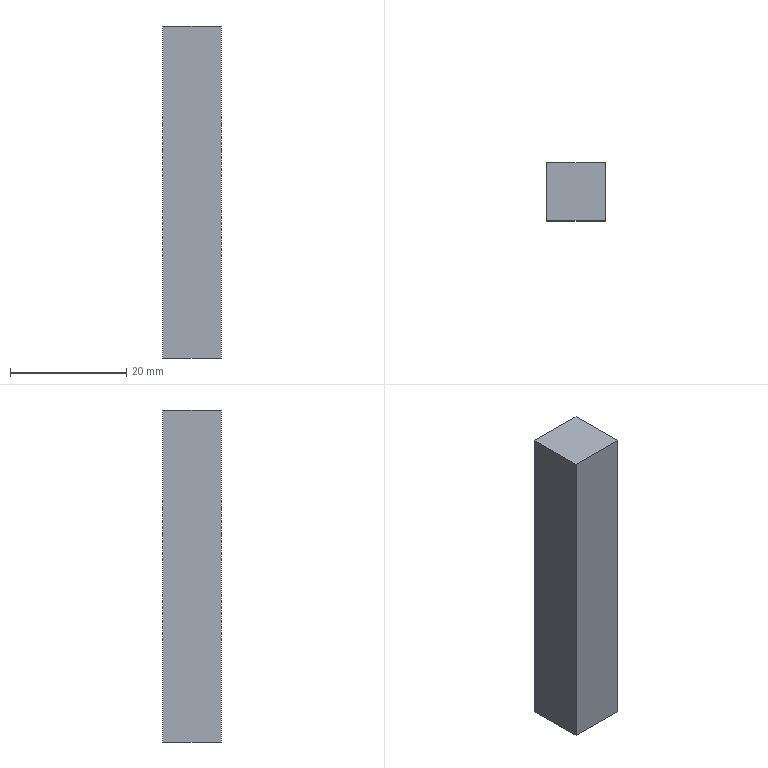Part | NX | features BREP 1 | 1 solid | 6 faces | box 10 x 10 x 57 mm | volume 5700 mm3 | plane 6
STEP:
#1=CARTESIAN_POINT('',(-1.25,10.55,-5.));
#2=VERTEX_POINT('',#1);
#3=CARTESIAN_POINT('',(-1.25,0.55,-5.));
#4=VERTEX_POINT('',#3);
#5=CARTESIAN_POINT('',(-1.25,10.55,-5.));
#6=DIRECTION('',(0.,-1.,0.));
#7=VECTOR('',#6,1000.);
#8=LINE('',#5,#7);
#9=EDGE_CURVE('',#2,#4,#8,.T.);
#10=ORIENTED_EDGE('',*,*,#9,.T.);
#11=CARTESIAN_POINT('',(-1.25,0.55,52.));
#12=VERTEX_POINT('',#11);
#13=CARTESIAN_POINT('',(-1.25,0.55,52.));
#14=DIRECTION('',(0.,0.,-1.));
#15=VECTOR('',#14,1000.);
#16=LINE('',#13,#15);
#17=EDGE_CURVE('',#12,#4,#16,.T.);
#18=ORIENTED_EDGE('',*,*,#17,.F.);
#19=CARTESIAN_POINT('',(-1.25,10.55,52.));
#20=VERTEX_POINT('',#19);
#21=CARTESIAN_POINT('',(-1.25,10.55,52.));
#22=DIRECTION('',(0.,-1.,0.));
#23=VECTOR('',#22,1000.);
#24=LINE('',#21,#23);
#25=EDGE_CURVE('',#20,#12,#24,.T.);
#26=ORIENTED_EDGE('',*,*,#25,.F.);
#27=CARTESIAN_POINT('',(-1.25,10.55,52.));
#28=DIRECTION('',(0.,0.,-1.));
#29=VECTOR('',#28,1000.);
#30=LINE('',#27,#29);
#31=EDGE_CURVE('',#20,#2,#30,.T.);
#32=ORIENTED_EDGE('',*,*,#31,.T.);
#33=EDGE_LOOP('',(#10,#18,#26,#32));
#34=FACE_BOUND('',#33,.T.);
#35=CARTESIAN_POINT('',(-1.25,10.55,52.));
#36=DIRECTION('',(1.,0.,0.));
#37=DIRECTION('',(0.,0.,1.));
#38=AXIS2_PLACEMENT_3D('',#35,#36,#37);
#39=PLANE('',#38);
#40=ADVANCED_FACE('',(#34),#39,.F.);
#41=CARTESIAN_POINT('',(8.75,0.55,-5.));
#42=VERTEX_POINT('',#41);
#43=CARTESIAN_POINT('',(-1.25,0.55,-5.));
#44=DIRECTION('',(1.,0.,0.));
#45=VECTOR('',#44,1000.);
#46=LINE('',#43,#45);
#47=EDGE_CURVE('',#4,#42,#46,.T.);
#48=ORIENTED_EDGE('',*,*,#47,.T.);
#49=CARTESIAN_POINT('',(8.75,0.55,52.));
#50=VERTEX_POINT('',#49);
#51=CARTESIAN_POINT('',(8.75,0.55,52.));
#52=DIRECTION('',(0.,0.,-1.));
#53=VECTOR('',#52,1000.);
#54=LINE('',#51,#53);
#55=EDGE_CURVE('',#50,#42,#54,.T.);
#56=ORIENTED_EDGE('',*,*,#55,.F.);
#57=CARTESIAN_POINT('',(-1.25,0.55,52.));
#58=DIRECTION('',(1.,0.,0.));
#59=VECTOR('',#58,1000.);
#60=LINE('',#57,#59);
#61=EDGE_CURVE('',#12,#50,#60,.T.);
#62=ORIENTED_EDGE('',*,*,#61,.F.);
#63=ORIENTED_EDGE('',*,*,#17,.T.);
#64=EDGE_LOOP('',(#48,#56,#62,#63));
#65=FACE_BOUND('',#64,.T.);
#66=CARTESIAN_POINT('',(-1.25,0.55,52.));
#67=DIRECTION('',(0.,1.,0.));
#68=DIRECTION('',(0.,0.,-1.));
#69=AXIS2_PLACEMENT_3D('',#66,#67,#68);
#70=PLANE('',#69);
#71=ADVANCED_FACE('',(#65),#70,.F.);
#72=CARTESIAN_POINT('',(8.75,10.55,-5.));
#73=VERTEX_POINT('',#72);
#74=CARTESIAN_POINT('',(8.75,0.55,-5.));
#75=DIRECTION('',(0.,1.,0.));
#76=VECTOR('',#75,1000.);
#77=LINE('',#74,#76);
#78=EDGE_CURVE('',#42,#73,#77,.T.);
#79=ORIENTED_EDGE('',*,*,#78,.T.);
#80=CARTESIAN_POINT('',(8.75,10.55,52.));
#81=VERTEX_POINT('',#80);
#82=CARTESIAN_POINT('',(8.75,10.55,52.));
#83=DIRECTION('',(0.,0.,-1.));
#84=VECTOR('',#83,1000.);
#85=LINE('',#82,#84);
#86=EDGE_CURVE('',#81,#73,#85,.T.);
#87=ORIENTED_EDGE('',*,*,#86,.F.);
#88=CARTESIAN_POINT('',(8.75,0.55,52.));
#89=DIRECTION('',(0.,1.,0.));
#90=VECTOR('',#89,1000.);
#91=LINE('',#88,#90);
#92=EDGE_CURVE('',#50,#81,#91,.T.);
#93=ORIENTED_EDGE('',*,*,#92,.F.);
#94=ORIENTED_EDGE('',*,*,#55,.T.);
#95=EDGE_LOOP('',(#79,#87,#93,#94));
#96=FACE_BOUND('',#95,.T.);
#97=CARTESIAN_POINT('',(8.75,0.55,52.));
#98=DIRECTION('',(-1.,0.,0.));
#99=DIRECTION('',(0.,0.,-1.));
#100=AXIS2_PLACEMENT_3D('',#97,#98,#99);
#101=PLANE('',#100);
#102=ADVANCED_FACE('',(#96),#101,.F.);
#103=CARTESIAN_POINT('',(8.75,10.55,-5.));
#104=DIRECTION('',(-1.,0.,0.));
#105=VECTOR('',#104,1000.);
#106=LINE('',#103,#105);
#107=EDGE_CURVE('',#73,#2,#106,.T.);
#108=ORIENTED_EDGE('',*,*,#107,.T.);
#109=ORIENTED_EDGE('',*,*,#31,.F.);
#110=CARTESIAN_POINT('',(8.75,10.55,52.));
#111=DIRECTION('',(-1.,0.,0.));
#112=VECTOR('',#111,1000.);
#113=LINE('',#110,#112);
#114=EDGE_CURVE('',#81,#20,#113,.T.);
#115=ORIENTED_EDGE('',*,*,#114,.F.);
#116=ORIENTED_EDGE('',*,*,#86,.T.);
#117=EDGE_LOOP('',(#108,#109,#115,#116));
#118=FACE_BOUND('',#117,.T.);
#119=CARTESIAN_POINT('',(8.75,10.55,52.));
#120=DIRECTION('',(0.,-1.,0.));
#121=DIRECTION('',(0.,0.,1.));
#122=AXIS2_PLACEMENT_3D('',#119,#120,#121);
#123=PLANE('',#122);
#124=ADVANCED_FACE('',(#118),#123,.F.);
#125=ORIENTED_EDGE('',*,*,#25,.T.);
#126=ORIENTED_EDGE('',*,*,#61,.T.);
#127=ORIENTED_EDGE('',*,*,#92,.T.);
#128=ORIENTED_EDGE('',*,*,#114,.T.);
#129=EDGE_LOOP('',(#125,#126,#127,#128));
#130=FACE_BOUND('',#129,.T.);
#131=CARTESIAN_POINT('',(0.,0.,52.));
#132=DIRECTION('',(0.,0.,1.));
#133=DIRECTION('',(-1.,0.,0.));
#134=AXIS2_PLACEMENT_3D('',#131,#132,#133);
#135=PLANE('',#134);
#136=ADVANCED_FACE('',(#130),#135,.T.);
#137=ORIENTED_EDGE('',*,*,#9,.F.);
#138=ORIENTED_EDGE('',*,*,#107,.F.);
#139=ORIENTED_EDGE('',*,*,#78,.F.);
#140=ORIENTED_EDGE('',*,*,#47,.F.);
#141=EDGE_LOOP('',(#137,#138,#139,#140));
#142=FACE_BOUND('',#141,.T.);
#143=CARTESIAN_POINT('',(0.,0.,-5.));
#144=DIRECTION('',(0.,0.,1.));
#145=DIRECTION('',(-1.,0.,0.));
#146=AXIS2_PLACEMENT_3D('',#143,#144,#145);
#147=PLANE('',#146);
#148=ADVANCED_FACE('',(#142),#147,.F.);
#149=CLOSED_SHELL('',(#40,#71,#102,#124,#136,#148));
#150=MANIFOLD_SOLID_BREP('',#149);
#151=(LENGTH_UNIT()NAMED_UNIT(*)SI_UNIT(.MILLI.,.METRE.));
#152=UNCERTAINTY_MEASURE_WITH_UNIT(LENGTH_MEASURE(0.00001),#151,'','');
#153=(NAMED_UNIT(*)PLANE_ANGLE_UNIT()SI_UNIT($,.RADIAN.));
#154=(NAMED_UNIT(*)SI_UNIT($,.STERADIAN.)SOLID_ANGLE_UNIT());
#155=(GEOMETRIC_REPRESENTATION_CONTEXT(3)GLOBAL_UNCERTAINTY_ASSIGNED_CONTEXT((#152))GLOBAL_UNIT_ASSIGNED_CONTEXT((#151,#153,#154))REPRESENTATION_CONTEXT('',''));
#156=ADVANCED_BREP_SHAPE_REPRESENTATION('',(#150),#155);